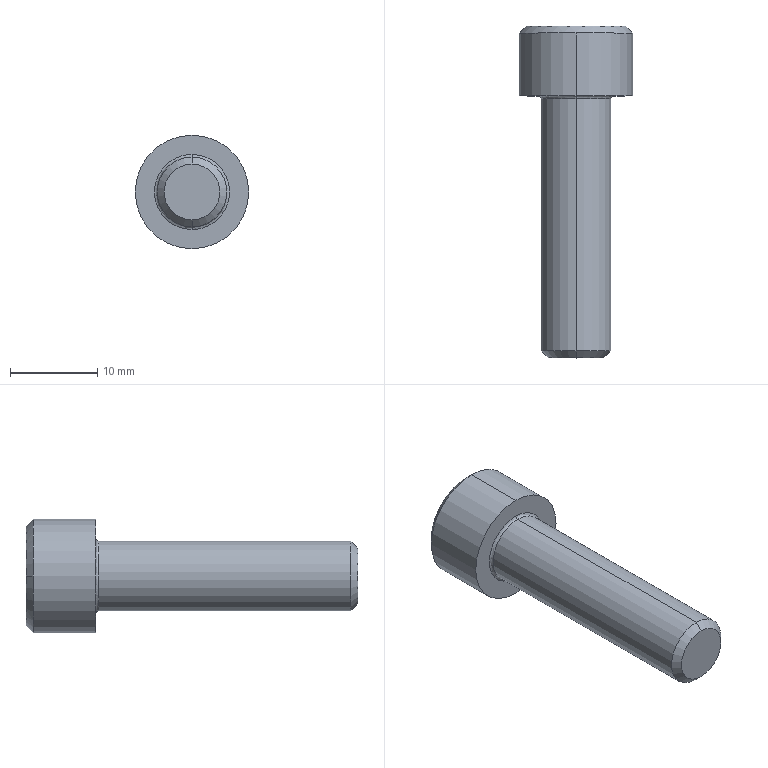Part | STEP file | 1 solid | 20 faces | box 13 x 38 x 13 mm | volume 2363 mm3 | plane 10 | cone 4 | cylinder 4 | spline 2 | commonest cylinder face diameters 8 x2 13 x2